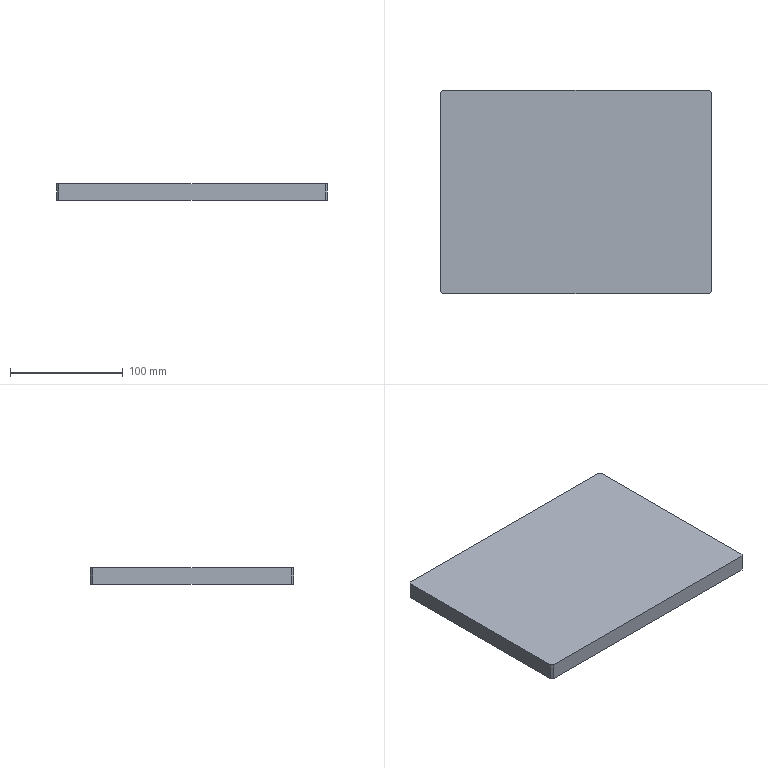Part | STEP file | 001-009-Riveting lower die base plate | 1 solid | 10 faces | box 240 x 180 x 15 mm | volume 647880 mm3 | plane 10
STEP:
#1=CARTESIAN_POINT('',(0.,0.,0.));
#2=DIRECTION('',(0.,0.,1.));
#3=DIRECTION('',(1.,0.,0.));
#4=AXIS2_PLACEMENT_3D('',#1,#2,#3);
#5=CARTESIAN_POINT('',(120.,-88.,0.));
#6=VERTEX_POINT('',#5);
#7=CARTESIAN_POINT('',(120.,88.,0.));
#8=VERTEX_POINT('',#7);
#9=CARTESIAN_POINT('',(120.,-90.,0.));
#10=DIRECTION('',(0.,1.,0.));
#11=VECTOR('',#10,1.);
#12=LINE('',#9,#11);
#13=CARTESIAN_POINT('',(120.,-90.,15.));
#14=DIRECTION('',(-1.,0.,0.));
#15=DIRECTION('',(0.,-1.,0.));
#16=AXIS2_PLACEMENT_3D('',#13,#14,#15);
#17=PLANE('',#16);
#18=CARTESIAN_POINT('',(0.,-15.));
#19=DIRECTION('',(-1.,0.));
#20=VECTOR('',#19,1.);
#21=LINE('',#18,#20);
#22=(GEOMETRIC_REPRESENTATION_CONTEXT(2)PARAMETRIC_REPRESENTATION_CONTEXT()REPRESENTATION_CONTEXT('',''));
#23=DEFINITIONAL_REPRESENTATION('',(#21),#22);
#24=PCURVE('',#17,#23);
#25=CARTESIAN_POINT('',(0.,0.,0.));
#26=DIRECTION('',(0.,0.,-1.));
#27=DIRECTION('',(-1.,0.,0.));
#28=AXIS2_PLACEMENT_3D('',#25,#26,#27);
#29=PLANE('',#28);
#30=CARTESIAN_POINT('',(-120.,-90.));
#31=DIRECTION('',(0.,1.));
#32=VECTOR('',#31,1.);
#33=LINE('',#30,#32);
#34=(GEOMETRIC_REPRESENTATION_CONTEXT(2)PARAMETRIC_REPRESENTATION_CONTEXT()REPRESENTATION_CONTEXT('',''));
#35=DEFINITIONAL_REPRESENTATION('',(#33),#34);
#36=PCURVE('',#29,#35);
#37=SURFACE_CURVE('',#12,(#24,#36),.PCURVE_S1.);
#38=EDGE_CURVE('',#6,#8,#37,.T.);
#39=ORIENTED_EDGE('',*,*,#38,.T.);
#40=CARTESIAN_POINT('',(120.,88.,15.));
#41=VERTEX_POINT('',#40);
#42=CARTESIAN_POINT('',(120.,88.,15.));
#43=DIRECTION('',(0.,0.,1.));
#44=VECTOR('',#43,1.);
#45=LINE('',#42,#44);
#46=CARTESIAN_POINT('',(-178.,0.));
#47=DIRECTION('',(0.,1.));
#48=VECTOR('',#47,1.);
#49=LINE('',#46,#48);
#50=(GEOMETRIC_REPRESENTATION_CONTEXT(2)PARAMETRIC_REPRESENTATION_CONTEXT()REPRESENTATION_CONTEXT('',''));
#51=DEFINITIONAL_REPRESENTATION('',(#49),#50);
#52=PCURVE('',#17,#51);
#53=CARTESIAN_POINT('',(118.,90.,15.));
#54=DIRECTION('',(-0.7071,-0.7071,0.));
#55=DIRECTION('',(0.,0.,-1.));
#56=AXIS2_PLACEMENT_3D('',#53,#54,#55);
#57=PLANE('',#56);
#58=CARTESIAN_POINT('',(0.,2.828));
#59=DIRECTION('',(-1.,0.));
#60=VECTOR('',#59,1.);
#61=LINE('',#58,#60);
#62=(GEOMETRIC_REPRESENTATION_CONTEXT(2)PARAMETRIC_REPRESENTATION_CONTEXT()REPRESENTATION_CONTEXT('',''));
#63=DEFINITIONAL_REPRESENTATION('',(#61),#62);
#64=PCURVE('',#57,#63);
#65=SURFACE_CURVE('',#45,(#52,#64),.PCURVE_S1.);
#66=EDGE_CURVE('',#8,#41,#65,.T.);
#67=ORIENTED_EDGE('',*,*,#66,.T.);
#68=CARTESIAN_POINT('',(120.,-88.,15.));
#69=VERTEX_POINT('',#68);
#70=CARTESIAN_POINT('',(120.,-90.,15.));
#71=DIRECTION('',(0.,1.,0.));
#72=VECTOR('',#71,1.);
#73=LINE('',#70,#72);
#74=CARTESIAN_POINT('',(0.,0.));
#75=DIRECTION('',(-1.,0.));
#76=VECTOR('',#75,1.);
#77=LINE('',#74,#76);
#78=(GEOMETRIC_REPRESENTATION_CONTEXT(2)PARAMETRIC_REPRESENTATION_CONTEXT()REPRESENTATION_CONTEXT('',''));
#79=DEFINITIONAL_REPRESENTATION('',(#77),#78);
#80=PCURVE('',#17,#79);
#81=CARTESIAN_POINT('',(0.,0.,15.));
#82=DIRECTION('',(0.,0.,-1.));
#83=DIRECTION('',(-1.,0.,0.));
#84=AXIS2_PLACEMENT_3D('',#81,#82,#83);
#85=PLANE('',#84);
#86=CARTESIAN_POINT('',(-120.,-90.));
#87=DIRECTION('',(0.,1.));
#88=VECTOR('',#87,1.);
#89=LINE('',#86,#88);
#90=(GEOMETRIC_REPRESENTATION_CONTEXT(2)PARAMETRIC_REPRESENTATION_CONTEXT()REPRESENTATION_CONTEXT('',''));
#91=DEFINITIONAL_REPRESENTATION('',(#89),#90);
#92=PCURVE('',#85,#91);
#93=SURFACE_CURVE('',#73,(#80,#92),.PCURVE_S1.);
#94=EDGE_CURVE('',#69,#41,#93,.T.);
#95=ORIENTED_EDGE('',*,*,#94,.F.);
#96=CARTESIAN_POINT('',(120.,-88.,15.));
#97=DIRECTION('',(0.,0.,-1.));
#98=VECTOR('',#97,1.);
#99=LINE('',#96,#98);
#100=CARTESIAN_POINT('',(-2.,0.));
#101=DIRECTION('',(0.,-1.));
#102=VECTOR('',#101,1.);
#103=LINE('',#100,#102);
#104=(GEOMETRIC_REPRESENTATION_CONTEXT(2)PARAMETRIC_REPRESENTATION_CONTEXT()REPRESENTATION_CONTEXT('',''));
#105=DEFINITIONAL_REPRESENTATION('',(#103),#104);
#106=PCURVE('',#17,#105);
#107=CARTESIAN_POINT('',(120.,-88.,15.));
#108=DIRECTION('',(-0.7071,0.7071,0.));
#109=DIRECTION('',(0.,0.,-1.));
#110=AXIS2_PLACEMENT_3D('',#107,#108,#109);
#111=PLANE('',#110);
#112=CARTESIAN_POINT('',(0.,0.));
#113=DIRECTION('',(1.,0.));
#114=VECTOR('',#113,1.);
#115=LINE('',#112,#114);
#116=(GEOMETRIC_REPRESENTATION_CONTEXT(2)PARAMETRIC_REPRESENTATION_CONTEXT()REPRESENTATION_CONTEXT('',''));
#117=DEFINITIONAL_REPRESENTATION('',(#115),#116);
#118=PCURVE('',#111,#117);
#119=SURFACE_CURVE('',#99,(#106,#118),.PCURVE_S1.);
#120=EDGE_CURVE('',#69,#6,#119,.T.);
#121=ORIENTED_EDGE('',*,*,#120,.T.);
#122=EDGE_LOOP('',(#39,#67,#95,#121));
#123=FACE_BOUND('',#122,.T.);
#124=ADVANCED_FACE('',(#123),#17,.F.);
#125=CARTESIAN_POINT('',(118.,90.,0.));
#126=VERTEX_POINT('',#125);
#127=CARTESIAN_POINT('',(-118.,90.,0.));
#128=VERTEX_POINT('',#127);
#129=CARTESIAN_POINT('',(-120.,90.,0.));
#130=DIRECTION('',(-1.,0.,0.));
#131=VECTOR('',#130,1.);
#132=LINE('',#129,#131);
#133=CARTESIAN_POINT('',(-120.,90.,15.));
#134=DIRECTION('',(0.,-1.,0.));
#135=DIRECTION('',(1.,0.,0.));
#136=AXIS2_PLACEMENT_3D('',#133,#134,#135);
#137=PLANE('',#136);
#138=CARTESIAN_POINT('',(0.,-15.));
#139=DIRECTION('',(-1.,0.));
#140=VECTOR('',#139,1.);
#141=LINE('',#138,#140);
#142=(GEOMETRIC_REPRESENTATION_CONTEXT(2)PARAMETRIC_REPRESENTATION_CONTEXT()REPRESENTATION_CONTEXT('',''));
#143=DEFINITIONAL_REPRESENTATION('',(#141),#142);
#144=PCURVE('',#137,#143);
#145=CARTESIAN_POINT('',(120.,90.));
#146=DIRECTION('',(1.,0.));
#147=VECTOR('',#146,1.);
#148=LINE('',#145,#147);
#149=(GEOMETRIC_REPRESENTATION_CONTEXT(2)PARAMETRIC_REPRESENTATION_CONTEXT()REPRESENTATION_CONTEXT('',''));
#150=DEFINITIONAL_REPRESENTATION('',(#148),#149);
#151=PCURVE('',#29,#150);
#152=SURFACE_CURVE('',#132,(#144,#151),.PCURVE_S1.);
#153=EDGE_CURVE('',#126,#128,#152,.T.);
#154=ORIENTED_EDGE('',*,*,#153,.T.);
#155=CARTESIAN_POINT('',(-118.,90.,15.));
#156=VERTEX_POINT('',#155);
#157=CARTESIAN_POINT('',(-118.,90.,15.));
#158=DIRECTION('',(0.,0.,1.));
#159=VECTOR('',#158,1.);
#160=LINE('',#157,#159);
#161=CARTESIAN_POINT('',(2.,0.));
#162=DIRECTION('',(0.,1.));
#163=VECTOR('',#162,1.);
#164=LINE('',#161,#163);
#165=(GEOMETRIC_REPRESENTATION_CONTEXT(2)PARAMETRIC_REPRESENTATION_CONTEXT()REPRESENTATION_CONTEXT('',''));
#166=DEFINITIONAL_REPRESENTATION('',(#164),#165);
#167=PCURVE('',#137,#166);
#168=CARTESIAN_POINT('',(-120.,88.,15.));
#169=DIRECTION('',(0.7071,-0.7071,0.));
#170=DIRECTION('',(0.,0.,-1.));
#171=AXIS2_PLACEMENT_3D('',#168,#169,#170);
#172=PLANE('',#171);
#173=CARTESIAN_POINT('',(0.,2.828));
#174=DIRECTION('',(-1.,0.));
#175=VECTOR('',#174,1.);
#176=LINE('',#173,#175);
#177=(GEOMETRIC_REPRESENTATION_CONTEXT(2)PARAMETRIC_REPRESENTATION_CONTEXT()REPRESENTATION_CONTEXT('',''));
#178=DEFINITIONAL_REPRESENTATION('',(#176),#177);
#179=PCURVE('',#172,#178);
#180=SURFACE_CURVE('',#160,(#167,#179),.PCURVE_S1.);
#181=EDGE_CURVE('',#128,#156,#180,.T.);
#182=ORIENTED_EDGE('',*,*,#181,.T.);
#183=CARTESIAN_POINT('',(118.,90.,15.));
#184=VERTEX_POINT('',#183);
#185=CARTESIAN_POINT('',(-120.,90.,15.));
#186=DIRECTION('',(-1.,0.,0.));
#187=VECTOR('',#186,1.);
#188=LINE('',#185,#187);
#189=CARTESIAN_POINT('',(0.,0.));
#190=DIRECTION('',(-1.,0.));
#191=VECTOR('',#190,1.);
#192=LINE('',#189,#191);
#193=(GEOMETRIC_REPRESENTATION_CONTEXT(2)PARAMETRIC_REPRESENTATION_CONTEXT()REPRESENTATION_CONTEXT('',''));
#194=DEFINITIONAL_REPRESENTATION('',(#192),#193);
#195=PCURVE('',#137,#194);
#196=CARTESIAN_POINT('',(120.,90.));
#197=DIRECTION('',(1.,0.));
#198=VECTOR('',#197,1.);
#199=LINE('',#196,#198);
#200=(GEOMETRIC_REPRESENTATION_CONTEXT(2)PARAMETRIC_REPRESENTATION_CONTEXT()REPRESENTATION_CONTEXT('',''));
#201=DEFINITIONAL_REPRESENTATION('',(#199),#200);
#202=PCURVE('',#85,#201);
#203=SURFACE_CURVE('',#188,(#195,#202),.PCURVE_S1.);
#204=EDGE_CURVE('',#184,#156,#203,.T.);
#205=ORIENTED_EDGE('',*,*,#204,.F.);
#206=CARTESIAN_POINT('',(118.,90.,15.));
#207=DIRECTION('',(0.,0.,-1.));
#208=VECTOR('',#207,1.);
#209=LINE('',#206,#208);
#210=CARTESIAN_POINT('',(238.,0.));
#211=DIRECTION('',(0.,-1.));
#212=VECTOR('',#211,1.);
#213=LINE('',#210,#212);
#214=(GEOMETRIC_REPRESENTATION_CONTEXT(2)PARAMETRIC_REPRESENTATION_CONTEXT()REPRESENTATION_CONTEXT('',''));
#215=DEFINITIONAL_REPRESENTATION('',(#213),#214);
#216=PCURVE('',#137,#215);
#217=CARTESIAN_POINT('',(0.,0.));
#218=DIRECTION('',(1.,0.));
#219=VECTOR('',#218,1.);
#220=LINE('',#217,#219);
#221=(GEOMETRIC_REPRESENTATION_CONTEXT(2)PARAMETRIC_REPRESENTATION_CONTEXT()REPRESENTATION_CONTEXT('',''));
#222=DEFINITIONAL_REPRESENTATION('',(#220),#221);
#223=PCURVE('',#57,#222);
#224=SURFACE_CURVE('',#209,(#216,#223),.PCURVE_S1.);
#225=EDGE_CURVE('',#184,#126,#224,.T.);
#226=ORIENTED_EDGE('',*,*,#225,.T.);
#227=EDGE_LOOP('',(#154,#182,#205,#226));
#228=FACE_BOUND('',#227,.T.);
#229=ADVANCED_FACE('',(#228),#137,.F.);
#230=CARTESIAN_POINT('',(-120.,88.,0.));
#231=VERTEX_POINT('',#230);
#232=CARTESIAN_POINT('',(-120.,-88.,0.));
#233=VERTEX_POINT('',#232);
#234=CARTESIAN_POINT('',(-120.,-90.,0.));
#235=DIRECTION('',(0.,-1.,0.));
#236=VECTOR('',#235,1.);
#237=LINE('',#234,#236);
#238=CARTESIAN_POINT('',(-120.,-90.,15.));
#239=DIRECTION('',(1.,0.,0.));
#240=DIRECTION('',(0.,0.,-1.));
#241=AXIS2_PLACEMENT_3D('',#238,#239,#240);
#242=PLANE('',#241);
#243=CARTESIAN_POINT('',(15.,0.));
#244=DIRECTION('',(0.,-1.));
#245=VECTOR('',#244,1.);
#246=LINE('',#243,#245);
#247=(GEOMETRIC_REPRESENTATION_CONTEXT(2)PARAMETRIC_REPRESENTATION_CONTEXT()REPRESENTATION_CONTEXT('',''));
#248=DEFINITIONAL_REPRESENTATION('',(#246),#247);
#249=PCURVE('',#242,#248);
#250=CARTESIAN_POINT('',(120.,-90.));
#251=DIRECTION('',(0.,-1.));
#252=VECTOR('',#251,1.);
#253=LINE('',#250,#252);
#254=(GEOMETRIC_REPRESENTATION_CONTEXT(2)PARAMETRIC_REPRESENTATION_CONTEXT()REPRESENTATION_CONTEXT('',''));
#255=DEFINITIONAL_REPRESENTATION('',(#253),#254);
#256=PCURVE('',#29,#255);
#257=SURFACE_CURVE('',#237,(#249,#256),.PCURVE_S1.);
#258=EDGE_CURVE('',#231,#233,#257,.T.);
#259=ORIENTED_EDGE('',*,*,#258,.T.);
#260=CARTESIAN_POINT('',(-120.,-88.,15.));
#261=VERTEX_POINT('',#260);
#262=CARTESIAN_POINT('',(-120.,-88.,15.));
#263=DIRECTION('',(0.,0.,1.));
#264=VECTOR('',#263,1.);
#265=LINE('',#262,#264);
#266=CARTESIAN_POINT('',(0.,2.));
#267=DIRECTION('',(-1.,0.));
#268=VECTOR('',#267,1.);
#269=LINE('',#266,#268);
#270=(GEOMETRIC_REPRESENTATION_CONTEXT(2)PARAMETRIC_REPRESENTATION_CONTEXT()REPRESENTATION_CONTEXT('',''));
#271=DEFINITIONAL_REPRESENTATION('',(#269),#270);
#272=PCURVE('',#242,#271);
#273=CARTESIAN_POINT('',(-118.,-90.,15.));
#274=DIRECTION('',(0.7071,0.7071,0.));
#275=DIRECTION('',(0.,0.,-1.));
#276=AXIS2_PLACEMENT_3D('',#273,#274,#275);
#277=PLANE('',#276);
#278=CARTESIAN_POINT('',(0.,2.828));
#279=DIRECTION('',(-1.,0.));
#280=VECTOR('',#279,1.);
#281=LINE('',#278,#280);
#282=(GEOMETRIC_REPRESENTATION_CONTEXT(2)PARAMETRIC_REPRESENTATION_CONTEXT()REPRESENTATION_CONTEXT('',''));
#283=DEFINITIONAL_REPRESENTATION('',(#281),#282);
#284=PCURVE('',#277,#283);
#285=SURFACE_CURVE('',#265,(#272,#284),.PCURVE_S1.);
#286=EDGE_CURVE('',#233,#261,#285,.T.);
#287=ORIENTED_EDGE('',*,*,#286,.T.);
#288=CARTESIAN_POINT('',(-120.,88.,15.));
#289=VERTEX_POINT('',#288);
#290=CARTESIAN_POINT('',(-120.,-90.,15.));
#291=DIRECTION('',(0.,-1.,0.));
#292=VECTOR('',#291,1.);
#293=LINE('',#290,#292);
#294=CARTESIAN_POINT('',(0.,0.));
#295=DIRECTION('',(0.,-1.));
#296=VECTOR('',#295,1.);
#297=LINE('',#294,#296);
#298=(GEOMETRIC_REPRESENTATION_CONTEXT(2)PARAMETRIC_REPRESENTATION_CONTEXT()REPRESENTATION_CONTEXT('',''));
#299=DEFINITIONAL_REPRESENTATION('',(#297),#298);
#300=PCURVE('',#242,#299);
#301=CARTESIAN_POINT('',(120.,-90.));
#302=DIRECTION('',(0.,-1.));
#303=VECTOR('',#302,1.);
#304=LINE('',#301,#303);
#305=(GEOMETRIC_REPRESENTATION_CONTEXT(2)PARAMETRIC_REPRESENTATION_CONTEXT()REPRESENTATION_CONTEXT('',''));
#306=DEFINITIONAL_REPRESENTATION('',(#304),#305);
#307=PCURVE('',#85,#306);
#308=SURFACE_CURVE('',#293,(#300,#307),.PCURVE_S1.);
#309=EDGE_CURVE('',#289,#261,#308,.T.);
#310=ORIENTED_EDGE('',*,*,#309,.F.);
#311=CARTESIAN_POINT('',(-120.,88.,15.));
#312=DIRECTION('',(0.,0.,-1.));
#313=VECTOR('',#312,1.);
#314=LINE('',#311,#313);
#315=CARTESIAN_POINT('',(0.,178.));
#316=DIRECTION('',(1.,0.));
#317=VECTOR('',#316,1.);
#318=LINE('',#315,#317);
#319=(GEOMETRIC_REPRESENTATION_CONTEXT(2)PARAMETRIC_REPRESENTATION_CONTEXT()REPRESENTATION_CONTEXT('',''));
#320=DEFINITIONAL_REPRESENTATION('',(#318),#319);
#321=PCURVE('',#242,#320);
#322=CARTESIAN_POINT('',(0.,0.));
#323=DIRECTION('',(1.,0.));
#324=VECTOR('',#323,1.);
#325=LINE('',#322,#324);
#326=(GEOMETRIC_REPRESENTATION_CONTEXT(2)PARAMETRIC_REPRESENTATION_CONTEXT()REPRESENTATION_CONTEXT('',''));
#327=DEFINITIONAL_REPRESENTATION('',(#325),#326);
#328=PCURVE('',#172,#327);
#329=SURFACE_CURVE('',#314,(#321,#328),.PCURVE_S1.);
#330=EDGE_CURVE('',#289,#231,#329,.T.);
#331=ORIENTED_EDGE('',*,*,#330,.T.);
#332=EDGE_LOOP('',(#259,#287,#310,#331));
#333=FACE_BOUND('',#332,.T.);
#334=ADVANCED_FACE('',(#333),#242,.F.);
#335=CARTESIAN_POINT('',(-118.,-90.,15.));
#336=VERTEX_POINT('',#335);
#337=CARTESIAN_POINT('',(118.,-90.,15.));
#338=VERTEX_POINT('',#337);
#339=CARTESIAN_POINT('',(-120.,-90.,15.));
#340=DIRECTION('',(1.,0.,0.));
#341=VECTOR('',#340,1.);
#342=LINE('',#339,#341);
#343=CARTESIAN_POINT('',(-120.,-90.,15.));
#344=DIRECTION('',(0.,1.,0.));
#345=DIRECTION('',(0.,0.,1.));
#346=AXIS2_PLACEMENT_3D('',#343,#344,#345);
#347=PLANE('',#346);
#348=CARTESIAN_POINT('',(0.,0.));
#349=DIRECTION('',(0.,1.));
#350=VECTOR('',#349,1.);
#351=LINE('',#348,#350);
#352=(GEOMETRIC_REPRESENTATION_CONTEXT(2)PARAMETRIC_REPRESENTATION_CONTEXT()REPRESENTATION_CONTEXT('',''));
#353=DEFINITIONAL_REPRESENTATION('',(#351),#352);
#354=PCURVE('',#347,#353);
#355=CARTESIAN_POINT('',(120.,-90.));
#356=DIRECTION('',(-1.,0.));
#357=VECTOR('',#356,1.);
#358=LINE('',#355,#357);
#359=(GEOMETRIC_REPRESENTATION_CONTEXT(2)PARAMETRIC_REPRESENTATION_CONTEXT()REPRESENTATION_CONTEXT('',''));
#360=DEFINITIONAL_REPRESENTATION('',(#358),#359);
#361=PCURVE('',#85,#360);
#362=SURFACE_CURVE('',#342,(#354,#361),.PCURVE_S1.);
#363=EDGE_CURVE('',#336,#338,#362,.T.);
#364=ORIENTED_EDGE('',*,*,#363,.F.);
#365=CARTESIAN_POINT('',(-118.,-90.,0.));
#366=VERTEX_POINT('',#365);
#367=CARTESIAN_POINT('',(-118.,-90.,15.));
#368=DIRECTION('',(0.,0.,-1.));
#369=VECTOR('',#368,1.);
#370=LINE('',#367,#369);
#371=CARTESIAN_POINT('',(0.,2.));
#372=DIRECTION('',(-1.,0.));
#373=VECTOR('',#372,1.);
#374=LINE('',#371,#373);
#375=(GEOMETRIC_REPRESENTATION_CONTEXT(2)PARAMETRIC_REPRESENTATION_CONTEXT()REPRESENTATION_CONTEXT('',''));
#376=DEFINITIONAL_REPRESENTATION('',(#374),#375);
#377=PCURVE('',#347,#376);
#378=CARTESIAN_POINT('',(0.,0.));
#379=DIRECTION('',(1.,0.));
#380=VECTOR('',#379,1.);
#381=LINE('',#378,#380);
#382=(GEOMETRIC_REPRESENTATION_CONTEXT(2)PARAMETRIC_REPRESENTATION_CONTEXT()REPRESENTATION_CONTEXT('',''));
#383=DEFINITIONAL_REPRESENTATION('',(#381),#382);
#384=PCURVE('',#277,#383);
#385=SURFACE_CURVE('',#370,(#377,#384),.PCURVE_S1.);
#386=EDGE_CURVE('',#336,#366,#385,.T.);
#387=ORIENTED_EDGE('',*,*,#386,.T.);
#388=CARTESIAN_POINT('',(118.,-90.,0.));
#389=VERTEX_POINT('',#388);
#390=CARTESIAN_POINT('',(-120.,-90.,0.));
#391=DIRECTION('',(1.,0.,0.));
#392=VECTOR('',#391,1.);
#393=LINE('',#390,#392);
#394=CARTESIAN_POINT('',(-15.,0.));
#395=DIRECTION('',(0.,1.));
#396=VECTOR('',#395,1.);
#397=LINE('',#394,#396);
#398=(GEOMETRIC_REPRESENTATION_CONTEXT(2)PARAMETRIC_REPRESENTATION_CONTEXT()REPRESENTATION_CONTEXT('',''));
#399=DEFINITIONAL_REPRESENTATION('',(#397),#398);
#400=PCURVE('',#347,#399);
#401=CARTESIAN_POINT('',(120.,-90.));
#402=DIRECTION('',(-1.,0.));
#403=VECTOR('',#402,1.);
#404=LINE('',#401,#403);
#405=(GEOMETRIC_REPRESENTATION_CONTEXT(2)PARAMETRIC_REPRESENTATION_CONTEXT()REPRESENTATION_CONTEXT('',''));
#406=DEFINITIONAL_REPRESENTATION('',(#404),#405);
#407=PCURVE('',#29,#406);
#408=SURFACE_CURVE('',#393,(#400,#407),.PCURVE_S1.);
#409=EDGE_CURVE('',#366,#389,#408,.T.);
#410=ORIENTED_EDGE('',*,*,#409,.T.);
#411=CARTESIAN_POINT('',(118.,-90.,15.));
#412=DIRECTION('',(0.,0.,1.));
#413=VECTOR('',#412,1.);
#414=LINE('',#411,#413);
#415=CARTESIAN_POINT('',(0.,238.));
#416=DIRECTION('',(1.,0.));
#417=VECTOR('',#416,1.);
#418=LINE('',#415,#417);
#419=(GEOMETRIC_REPRESENTATION_CONTEXT(2)PARAMETRIC_REPRESENTATION_CONTEXT()REPRESENTATION_CONTEXT('',''));
#420=DEFINITIONAL_REPRESENTATION('',(#418),#419);
#421=PCURVE('',#347,#420);
#422=CARTESIAN_POINT('',(0.,2.828));
#423=DIRECTION('',(-1.,0.));
#424=VECTOR('',#423,1.);
#425=LINE('',#422,#424);
#426=(GEOMETRIC_REPRESENTATION_CONTEXT(2)PARAMETRIC_REPRESENTATION_CONTEXT()REPRESENTATION_CONTEXT('',''));
#427=DEFINITIONAL_REPRESENTATION('',(#425),#426);
#428=PCURVE('',#111,#427);
#429=SURFACE_CURVE('',#414,(#421,#428),.PCURVE_S1.);
#430=EDGE_CURVE('',#389,#338,#429,.T.);
#431=ORIENTED_EDGE('',*,*,#430,.T.);
#432=EDGE_LOOP('',(#364,#387,#410,#431));
#433=FACE_BOUND('',#432,.T.);
#434=ADVANCED_FACE('',(#433),#347,.F.);
#435=ORIENTED_EDGE('',*,*,#309,.T.);
#436=CARTESIAN_POINT('',(-118.,-90.,15.));
#437=DIRECTION('',(0.7071,-0.7071,0.));
#438=VECTOR('',#437,1.);
#439=LINE('',#436,#438);
#440=CARTESIAN_POINT('',(118.,-90.));
#441=DIRECTION('',(-0.7071,-0.7071));
#442=VECTOR('',#441,1.);
#443=LINE('',#440,#442);
#444=(GEOMETRIC_REPRESENTATION_CONTEXT(2)PARAMETRIC_REPRESENTATION_CONTEXT()REPRESENTATION_CONTEXT('',''));
#445=DEFINITIONAL_REPRESENTATION('',(#443),#444);
#446=PCURVE('',#85,#445);
#447=CARTESIAN_POINT('',(0.,0.));
#448=DIRECTION('',(0.,-1.));
#449=VECTOR('',#448,1.);
#450=LINE('',#447,#449);
#451=(GEOMETRIC_REPRESENTATION_CONTEXT(2)PARAMETRIC_REPRESENTATION_CONTEXT()REPRESENTATION_CONTEXT('',''));
#452=DEFINITIONAL_REPRESENTATION('',(#450),#451);
#453=PCURVE('',#277,#452);
#454=SURFACE_CURVE('',#439,(#446,#453),.PCURVE_S1.);
#455=EDGE_CURVE('',#261,#336,#454,.T.);
#456=ORIENTED_EDGE('',*,*,#455,.T.);
#457=ORIENTED_EDGE('',*,*,#363,.T.);
#458=CARTESIAN_POINT('',(120.,-88.,15.));
#459=DIRECTION('',(0.7071,0.7071,0.));
#460=VECTOR('',#459,1.);
#461=LINE('',#458,#460);
#462=CARTESIAN_POINT('',(-120.,-88.));
#463=DIRECTION('',(-0.7071,0.7071));
#464=VECTOR('',#463,1.);
#465=LINE('',#462,#464);
#466=(GEOMETRIC_REPRESENTATION_CONTEXT(2)PARAMETRIC_REPRESENTATION_CONTEXT()REPRESENTATION_CONTEXT('',''));
#467=DEFINITIONAL_REPRESENTATION('',(#465),#466);
#468=PCURVE('',#85,#467);
#469=CARTESIAN_POINT('',(0.,0.));
#470=DIRECTION('',(0.,-1.));
#471=VECTOR('',#470,1.);
#472=LINE('',#469,#471);
#473=(GEOMETRIC_REPRESENTATION_CONTEXT(2)PARAMETRIC_REPRESENTATION_CONTEXT()REPRESENTATION_CONTEXT('',''));
#474=DEFINITIONAL_REPRESENTATION('',(#472),#473);
#475=PCURVE('',#111,#474);
#476=SURFACE_CURVE('',#461,(#468,#475),.PCURVE_S1.);
#477=EDGE_CURVE('',#338,#69,#476,.T.);
#478=ORIENTED_EDGE('',*,*,#477,.T.);
#479=ORIENTED_EDGE('',*,*,#94,.T.);
#480=CARTESIAN_POINT('',(118.,90.,15.));
#481=DIRECTION('',(-0.7071,0.7071,0.));
#482=VECTOR('',#481,1.);
#483=LINE('',#480,#482);
#484=CARTESIAN_POINT('',(-118.,90.));
#485=DIRECTION('',(0.7071,0.7071));
#486=VECTOR('',#485,1.);
#487=LINE('',#484,#486);
#488=(GEOMETRIC_REPRESENTATION_CONTEXT(2)PARAMETRIC_REPRESENTATION_CONTEXT()REPRESENTATION_CONTEXT('',''));
#489=DEFINITIONAL_REPRESENTATION('',(#487),#488);
#490=PCURVE('',#85,#489);
#491=CARTESIAN_POINT('',(0.,0.));
#492=DIRECTION('',(0.,-1.));
#493=VECTOR('',#492,1.);
#494=LINE('',#491,#493);
#495=(GEOMETRIC_REPRESENTATION_CONTEXT(2)PARAMETRIC_REPRESENTATION_CONTEXT()REPRESENTATION_CONTEXT('',''));
#496=DEFINITIONAL_REPRESENTATION('',(#494),#495);
#497=PCURVE('',#57,#496);
#498=SURFACE_CURVE('',#483,(#490,#497),.PCURVE_S1.);
#499=EDGE_CURVE('',#41,#184,#498,.T.);
#500=ORIENTED_EDGE('',*,*,#499,.T.);
#501=ORIENTED_EDGE('',*,*,#204,.T.);
#502=CARTESIAN_POINT('',(-120.,88.,15.));
#503=DIRECTION('',(-0.7071,-0.7071,0.));
#504=VECTOR('',#503,1.);
#505=LINE('',#502,#504);
#506=CARTESIAN_POINT('',(120.,88.));
#507=DIRECTION('',(0.7071,-0.7071));
#508=VECTOR('',#507,1.);
#509=LINE('',#506,#508);
#510=(GEOMETRIC_REPRESENTATION_CONTEXT(2)PARAMETRIC_REPRESENTATION_CONTEXT()REPRESENTATION_CONTEXT('',''));
#511=DEFINITIONAL_REPRESENTATION('',(#509),#510);
#512=PCURVE('',#85,#511);
#513=CARTESIAN_POINT('',(0.,0.));
#514=DIRECTION('',(0.,-1.));
#515=VECTOR('',#514,1.);
#516=LINE('',#513,#515);
#517=(GEOMETRIC_REPRESENTATION_CONTEXT(2)PARAMETRIC_REPRESENTATION_CONTEXT()REPRESENTATION_CONTEXT('',''));
#518=DEFINITIONAL_REPRESENTATION('',(#516),#517);
#519=PCURVE('',#172,#518);
#520=SURFACE_CURVE('',#505,(#512,#519),.PCURVE_S1.);
#521=EDGE_CURVE('',#156,#289,#520,.T.);
#522=ORIENTED_EDGE('',*,*,#521,.T.);
#523=EDGE_LOOP('',(#435,#456,#457,#478,#479,#500,#501,#522));
#524=FACE_BOUND('',#523,.T.);
#525=ADVANCED_FACE('',(#524),#85,.F.);
#526=ORIENTED_EDGE('',*,*,#409,.F.);
#527=CARTESIAN_POINT('',(-104.,-104.,0.));
#528=DIRECTION('',(-0.7071,0.7071,0.));
#529=VECTOR('',#528,1.);
#530=LINE('',#527,#529);
#531=CARTESIAN_POINT('',(104.,-104.));
#532=DIRECTION('',(0.7071,0.7071));
#533=VECTOR('',#532,1.);
#534=LINE('',#531,#533);
#535=(GEOMETRIC_REPRESENTATION_CONTEXT(2)PARAMETRIC_REPRESENTATION_CONTEXT()REPRESENTATION_CONTEXT('',''));
#536=DEFINITIONAL_REPRESENTATION('',(#534),#535);
#537=PCURVE('',#29,#536);
#538=CARTESIAN_POINT('',(15.,-19.799));
#539=DIRECTION('',(0.,1.));
#540=VECTOR('',#539,1.);
#541=LINE('',#538,#540);
#542=(GEOMETRIC_REPRESENTATION_CONTEXT(2)PARAMETRIC_REPRESENTATION_CONTEXT()REPRESENTATION_CONTEXT('',''));
#543=DEFINITIONAL_REPRESENTATION('',(#541),#542);
#544=PCURVE('',#277,#543);
#545=SURFACE_CURVE('',#530,(#537,#544),.PCURVE_S1.);
#546=EDGE_CURVE('',#366,#233,#545,.T.);
#547=ORIENTED_EDGE('',*,*,#546,.T.);
#548=ORIENTED_EDGE('',*,*,#258,.F.);
#549=CARTESIAN_POINT('',(-104.,104.,0.));
#550=DIRECTION('',(0.7071,0.7071,0.));
#551=VECTOR('',#550,1.);
#552=LINE('',#549,#551);
#553=CARTESIAN_POINT('',(104.,104.));
#554=DIRECTION('',(-0.7071,0.7071));
#555=VECTOR('',#554,1.);
#556=LINE('',#553,#555);
#557=(GEOMETRIC_REPRESENTATION_CONTEXT(2)PARAMETRIC_REPRESENTATION_CONTEXT()REPRESENTATION_CONTEXT('',''));
#558=DEFINITIONAL_REPRESENTATION('',(#556),#557);
#559=PCURVE('',#29,#558);
#560=CARTESIAN_POINT('',(15.,22.627));
#561=DIRECTION('',(0.,1.));
#562=VECTOR('',#561,1.);
#563=LINE('',#560,#562);
#564=(GEOMETRIC_REPRESENTATION_CONTEXT(2)PARAMETRIC_REPRESENTATION_CONTEXT()REPRESENTATION_CONTEXT('',''));
#565=DEFINITIONAL_REPRESENTATION('',(#563),#564);
#566=PCURVE('',#172,#565);
#567=SURFACE_CURVE('',#552,(#559,#566),.PCURVE_S1.);
#568=EDGE_CURVE('',#231,#128,#567,.T.);
#569=ORIENTED_EDGE('',*,*,#568,.T.);
#570=ORIENTED_EDGE('',*,*,#153,.F.);
#571=CARTESIAN_POINT('',(104.,104.,0.));
#572=DIRECTION('',(0.7071,-0.7071,0.));
#573=VECTOR('',#572,1.);
#574=LINE('',#571,#573);
#575=CARTESIAN_POINT('',(-104.,104.));
#576=DIRECTION('',(-0.7071,-0.7071));
#577=VECTOR('',#576,1.);
#578=LINE('',#575,#577);
#579=(GEOMETRIC_REPRESENTATION_CONTEXT(2)PARAMETRIC_REPRESENTATION_CONTEXT()REPRESENTATION_CONTEXT('',''));
#580=DEFINITIONAL_REPRESENTATION('',(#578),#579);
#581=PCURVE('',#29,#580);
#582=CARTESIAN_POINT('',(15.,-19.799));
#583=DIRECTION('',(0.,1.));
#584=VECTOR('',#583,1.);
#585=LINE('',#582,#584);
#586=(GEOMETRIC_REPRESENTATION_CONTEXT(2)PARAMETRIC_REPRESENTATION_CONTEXT()REPRESENTATION_CONTEXT('',''));
#587=DEFINITIONAL_REPRESENTATION('',(#585),#586);
#588=PCURVE('',#57,#587);
#589=SURFACE_CURVE('',#574,(#581,#588),.PCURVE_S1.);
#590=EDGE_CURVE('',#126,#8,#589,.T.);
#591=ORIENTED_EDGE('',*,*,#590,.T.);
#592=ORIENTED_EDGE('',*,*,#38,.F.);
#593=CARTESIAN_POINT('',(104.,-104.,0.));
#594=DIRECTION('',(-0.7071,-0.7071,0.));
#595=VECTOR('',#594,1.);
#596=LINE('',#593,#595);
#597=CARTESIAN_POINT('',(-104.,-104.));
#598=DIRECTION('',(0.7071,-0.7071));
#599=VECTOR('',#598,1.);
#600=LINE('',#597,#599);
#601=(GEOMETRIC_REPRESENTATION_CONTEXT(2)PARAMETRIC_REPRESENTATION_CONTEXT()REPRESENTATION_CONTEXT('',''));
#602=DEFINITIONAL_REPRESENTATION('',(#600),#601);
#603=PCURVE('',#29,#602);
#604=CARTESIAN_POINT('',(15.,22.627));
#605=DIRECTION('',(0.,1.));
#606=VECTOR('',#605,1.);
#607=LINE('',#604,#606);
#608=(GEOMETRIC_REPRESENTATION_CONTEXT(2)PARAMETRIC_REPRESENTATION_CONTEXT()REPRESENTATION_CONTEXT('',''));
#609=DEFINITIONAL_REPRESENTATION('',(#607),#608);
#610=PCURVE('',#111,#609);
#611=SURFACE_CURVE('',#596,(#603,#610),.PCURVE_S1.);
#612=EDGE_CURVE('',#6,#389,#611,.T.);
#613=ORIENTED_EDGE('',*,*,#612,.T.);
#614=EDGE_LOOP('',(#526,#547,#548,#569,#570,#591,#592,#613));
#615=FACE_BOUND('',#614,.T.);
#616=ADVANCED_FACE('',(#615),#29,.T.);
#617=ORIENTED_EDGE('',*,*,#455,.F.);
#618=ORIENTED_EDGE('',*,*,#286,.F.);
#619=ORIENTED_EDGE('',*,*,#546,.F.);
#620=ORIENTED_EDGE('',*,*,#386,.F.);
#621=EDGE_LOOP('',(#617,#618,#619,#620));
#622=FACE_BOUND('',#621,.T.);
#623=ADVANCED_FACE('',(#622),#277,.F.);
#624=ORIENTED_EDGE('',*,*,#521,.F.);
#625=ORIENTED_EDGE('',*,*,#181,.F.);
#626=ORIENTED_EDGE('',*,*,#568,.F.);
#627=ORIENTED_EDGE('',*,*,#330,.F.);
#628=EDGE_LOOP('',(#624,#625,#626,#627));
#629=FACE_BOUND('',#628,.T.);
#630=ADVANCED_FACE('',(#629),#172,.F.);
#631=ORIENTED_EDGE('',*,*,#499,.F.);
#632=ORIENTED_EDGE('',*,*,#66,.F.);
#633=ORIENTED_EDGE('',*,*,#590,.F.);
#634=ORIENTED_EDGE('',*,*,#225,.F.);
#635=EDGE_LOOP('',(#631,#632,#633,#634));
#636=FACE_BOUND('',#635,.T.);
#637=ADVANCED_FACE('',(#636),#57,.F.);
#638=ORIENTED_EDGE('',*,*,#477,.F.);
#639=ORIENTED_EDGE('',*,*,#430,.F.);
#640=ORIENTED_EDGE('',*,*,#612,.F.);
#641=ORIENTED_EDGE('',*,*,#120,.F.);
#642=EDGE_LOOP('',(#638,#639,#640,#641));
#643=FACE_BOUND('',#642,.T.);
#644=ADVANCED_FACE('',(#643),#111,.F.);
#645=CLOSED_SHELL('',(#124,#229,#334,#434,#525,#616,#623,#630,#637,#644));
#646=MANIFOLD_SOLID_BREP('',#645);
#647=(LENGTH_UNIT()NAMED_UNIT(*)SI_UNIT(.MILLI.,.METRE.));
#648=UNCERTAINTY_MEASURE_WITH_UNIT(LENGTH_MEASURE(0.0000001),#647,'','');
#649=(NAMED_UNIT(*)PLANE_ANGLE_UNIT()SI_UNIT($,.RADIAN.));
#650=(NAMED_UNIT(*)SI_UNIT($,.STERADIAN.)SOLID_ANGLE_UNIT());
#651=(GEOMETRIC_REPRESENTATION_CONTEXT(3)GLOBAL_UNCERTAINTY_ASSIGNED_CONTEXT((#648))GLOBAL_UNIT_ASSIGNED_CONTEXT((#647,#649,#650))REPRESENTATION_CONTEXT('',''));
#652=ADVANCED_BREP_SHAPE_REPRESENTATION('',(#4,#646),#651);